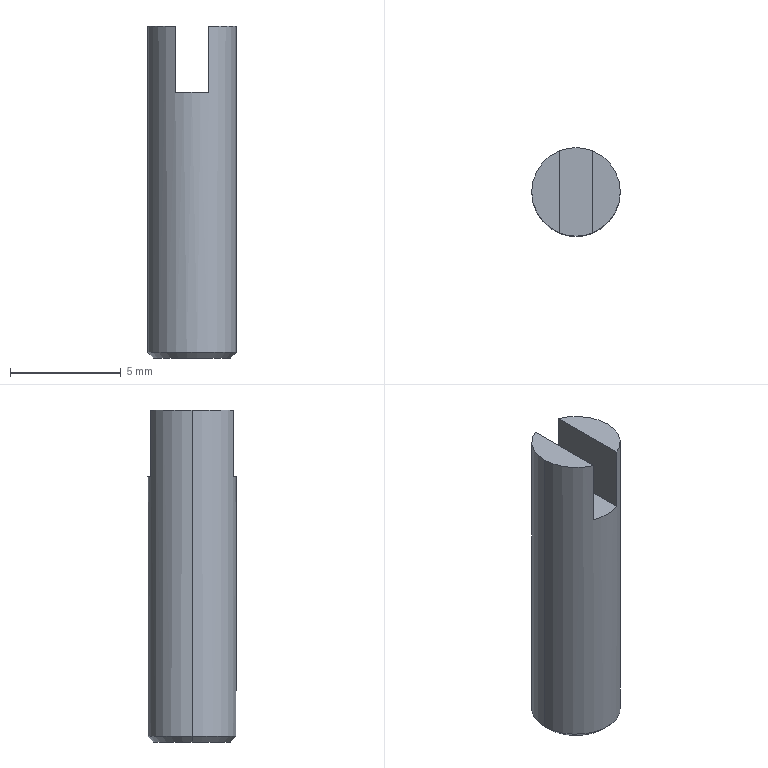Part | SolidWorks | features BaseBody 1 | 1 solid | 10 faces | box 4 x 4 x 15 mm | volume 170.55 mm3 | plane 6 | cone 2 | cylinder 2 | commonest cylinder face diameters 4 x2
STEP:
#1=CARTESIAN_POINT('',(-1.75,0.,0.));
#2=VERTEX_POINT('',#1);
#3=CARTESIAN_POINT('',(1.75,0.,0.));
#4=VERTEX_POINT('',#3);
#5=CARTESIAN_POINT('',(0.,0.,0.));
#6=DIRECTION('',(0.,0.,1.));
#7=DIRECTION('',(-1.,0.,0.));
#8=AXIS2_PLACEMENT_3D('',#5,#6,#7);
#9=CIRCLE('',#8,1.75);
#10=EDGE_CURVE('',#2,#4,#9,.T.);
#11=ORIENTED_EDGE('',*,*,#10,.T.);
#12=CARTESIAN_POINT('',(2.,0.,0.25));
#13=VERTEX_POINT('',#12);
#14=CARTESIAN_POINT('',(1.875,0.,0.125));
#15=DIRECTION('',(0.7071,0.,0.7071));
#16=VECTOR('',#15,1000.);
#17=LINE('',#14,#16);
#18=EDGE_CURVE('',#4,#13,#17,.T.);
#19=ORIENTED_EDGE('',*,*,#18,.T.);
#20=CARTESIAN_POINT('',(-2.,0.,0.25));
#21=VERTEX_POINT('',#20);
#22=CARTESIAN_POINT('',(0.,0.,0.25));
#23=DIRECTION('',(0.,0.,-1.));
#24=DIRECTION('',(-1.,0.,0.));
#25=AXIS2_PLACEMENT_3D('',#22,#23,#24);
#26=CIRCLE('',#25,2.);
#27=EDGE_CURVE('',#13,#21,#26,.T.);
#28=ORIENTED_EDGE('',*,*,#27,.T.);
#29=CARTESIAN_POINT('',(-1.875,0.,0.125));
#30=DIRECTION('',(-0.7071,0.,0.7071));
#31=VECTOR('',#30,1000.);
#32=LINE('',#29,#31);
#33=EDGE_CURVE('',#2,#21,#32,.T.);
#34=ORIENTED_EDGE('',*,*,#33,.F.);
#35=EDGE_LOOP('',(#11,#19,#28,#34));
#36=FACE_OUTER_BOUND('',#35,.T.);
#37=CARTESIAN_POINT('',(0.,0.,0.125));
#38=DIRECTION('',(0.,0.,1.));
#39=DIRECTION('',(-1.,0.,0.));
#40=AXIS2_PLACEMENT_3D('',#37,#38,#39);
#41=CONICAL_SURFACE('',#40,1.875,0.7854);
#42=ADVANCED_FACE('',(#36),#41,.T.);
#43=CARTESIAN_POINT('',(2.,0.,15.));
#44=VERTEX_POINT('',#43);
#45=CARTESIAN_POINT('',(0.75,1.854,15.));
#46=VERTEX_POINT('',#45);
#47=CARTESIAN_POINT('',(0.,0.,15.));
#48=DIRECTION('',(0.,0.,1.));
#49=DIRECTION('',(-1.,0.,0.));
#50=AXIS2_PLACEMENT_3D('',#47,#48,#49);
#51=CIRCLE('',#50,2.);
#52=EDGE_CURVE('',#44,#46,#51,.T.);
#53=ORIENTED_EDGE('',*,*,#52,.F.);
#54=CARTESIAN_POINT('',(2.,0.,0.));
#55=DIRECTION('',(0.,0.,-1.));
#56=VECTOR('',#55,1000.);
#57=LINE('',#54,#56);
#58=EDGE_CURVE('',#44,#13,#57,.T.);
#59=ORIENTED_EDGE('',*,*,#58,.T.);
#60=CARTESIAN_POINT('',(0.,0.,0.25));
#61=DIRECTION('',(0.,0.,-1.));
#62=DIRECTION('',(-1.,0.,0.));
#63=AXIS2_PLACEMENT_3D('',#60,#61,#62);
#64=CIRCLE('',#63,2.);
#65=EDGE_CURVE('',#21,#13,#64,.T.);
#66=ORIENTED_EDGE('',*,*,#65,.F.);
#67=CARTESIAN_POINT('',(-2.,0.,15.));
#68=VERTEX_POINT('',#67);
#69=CARTESIAN_POINT('',(-2.,0.,0.));
#70=DIRECTION('',(0.,0.,-1.));
#71=VECTOR('',#70,1000.);
#72=LINE('',#69,#71);
#73=EDGE_CURVE('',#68,#21,#72,.T.);
#74=ORIENTED_EDGE('',*,*,#73,.F.);
#75=CARTESIAN_POINT('',(-0.75,1.854,15.));
#76=VERTEX_POINT('',#75);
#77=CARTESIAN_POINT('',(0.,0.,15.));
#78=DIRECTION('',(0.,0.,1.));
#79=DIRECTION('',(-1.,0.,0.));
#80=AXIS2_PLACEMENT_3D('',#77,#78,#79);
#81=CIRCLE('',#80,2.);
#82=EDGE_CURVE('',#76,#68,#81,.T.);
#83=ORIENTED_EDGE('',*,*,#82,.F.);
#84=CARTESIAN_POINT('',(-0.75,1.854,12.));
#85=VERTEX_POINT('',#84);
#86=CARTESIAN_POINT('',(-0.75,1.854,0.));
#87=DIRECTION('',(0.,0.,-1.));
#88=VECTOR('',#87,1000.);
#89=LINE('',#86,#88);
#90=EDGE_CURVE('',#76,#85,#89,.T.);
#91=ORIENTED_EDGE('',*,*,#90,.T.);
#92=CARTESIAN_POINT('',(0.75,1.854,12.));
#93=VERTEX_POINT('',#92);
#94=CARTESIAN_POINT('',(0.,0.,12.));
#95=DIRECTION('',(0.,0.,-1.));
#96=DIRECTION('',(-1.,0.,0.));
#97=AXIS2_PLACEMENT_3D('',#94,#95,#96);
#98=CIRCLE('',#97,2.);
#99=EDGE_CURVE('',#85,#93,#98,.T.);
#100=ORIENTED_EDGE('',*,*,#99,.T.);
#101=CARTESIAN_POINT('',(0.75,1.854,0.));
#102=DIRECTION('',(0.,0.,1.));
#103=VECTOR('',#102,1000.);
#104=LINE('',#101,#103);
#105=EDGE_CURVE('',#93,#46,#104,.T.);
#106=ORIENTED_EDGE('',*,*,#105,.T.);
#107=EDGE_LOOP('',(#53,#59,#66,#74,#83,#91,#100,#106));
#108=FACE_OUTER_BOUND('',#107,.T.);
#109=CARTESIAN_POINT('',(0.,0.,0.));
#110=DIRECTION('',(0.,0.,-1.));
#111=DIRECTION('',(-1.,0.,0.));
#112=AXIS2_PLACEMENT_3D('',#109,#110,#111);
#113=CYLINDRICAL_SURFACE('',#112,2.);
#114=ADVANCED_FACE('',(#108),#113,.T.);
#115=ORIENTED_EDGE('',*,*,#10,.F.);
#116=CARTESIAN_POINT('',(0.,0.,0.));
#117=DIRECTION('',(0.,0.,1.));
#118=DIRECTION('',(-1.,0.,0.));
#119=AXIS2_PLACEMENT_3D('',#116,#117,#118);
#120=CIRCLE('',#119,1.75);
#121=EDGE_CURVE('',#4,#2,#120,.T.);
#122=ORIENTED_EDGE('',*,*,#121,.F.);
#123=EDGE_LOOP('',(#115,#122));
#124=FACE_OUTER_BOUND('',#123,.T.);
#125=CARTESIAN_POINT('',(0.,0.,0.));
#126=DIRECTION('',(0.,0.,1.));
#127=DIRECTION('',(1.,0.,0.));
#128=AXIS2_PLACEMENT_3D('',#125,#126,#127);
#129=PLANE('',#128);
#130=ADVANCED_FACE('',(#124),#129,.F.);
#131=CARTESIAN_POINT('',(-0.75,-1.854,12.));
#132=VERTEX_POINT('',#131);
#133=CARTESIAN_POINT('',(-0.75,-1.854,15.));
#134=VERTEX_POINT('',#133);
#135=CARTESIAN_POINT('',(-0.75,-1.854,0.));
#136=DIRECTION('',(0.,0.,1.));
#137=VECTOR('',#136,1000.);
#138=LINE('',#135,#137);
#139=EDGE_CURVE('',#132,#134,#138,.T.);
#140=ORIENTED_EDGE('',*,*,#139,.F.);
#141=CARTESIAN_POINT('',(-0.75,-2.,12.));
#142=DIRECTION('',(0.,1.,0.));
#143=VECTOR('',#142,1000.);
#144=LINE('',#141,#143);
#145=EDGE_CURVE('',#132,#85,#144,.T.);
#146=ORIENTED_EDGE('',*,*,#145,.T.);
#147=ORIENTED_EDGE('',*,*,#90,.F.);
#148=CARTESIAN_POINT('',(-0.75,-1.,15.));
#149=DIRECTION('',(0.,1.,0.));
#150=VECTOR('',#149,1000.);
#151=LINE('',#148,#150);
#152=EDGE_CURVE('',#134,#76,#151,.T.);
#153=ORIENTED_EDGE('',*,*,#152,.F.);
#154=EDGE_LOOP('',(#140,#146,#147,#153));
#155=FACE_OUTER_BOUND('',#154,.T.);
#156=CARTESIAN_POINT('',(-0.75,-2.,15.));
#157=DIRECTION('',(-1.,0.,0.));
#158=DIRECTION('',(0.,1.,0.));
#159=AXIS2_PLACEMENT_3D('',#156,#157,#158);
#160=PLANE('',#159);
#161=ADVANCED_FACE('',(#155),#160,.F.);
#162=CARTESIAN_POINT('',(0.75,-1.854,12.));
#163=VERTEX_POINT('',#162);
#164=CARTESIAN_POINT('',(0.,0.,12.));
#165=DIRECTION('',(0.,0.,-1.));
#166=DIRECTION('',(-1.,0.,0.));
#167=AXIS2_PLACEMENT_3D('',#164,#165,#166);
#168=CIRCLE('',#167,2.);
#169=EDGE_CURVE('',#163,#132,#168,.T.);
#170=ORIENTED_EDGE('',*,*,#169,.F.);
#171=CARTESIAN_POINT('',(0.75,2.,12.));
#172=DIRECTION('',(0.,-1.,0.));
#173=VECTOR('',#172,1000.);
#174=LINE('',#171,#173);
#175=EDGE_CURVE('',#93,#163,#174,.T.);
#176=ORIENTED_EDGE('',*,*,#175,.F.);
#177=ORIENTED_EDGE('',*,*,#99,.F.);
#178=ORIENTED_EDGE('',*,*,#145,.F.);
#179=EDGE_LOOP('',(#170,#176,#177,#178));
#180=FACE_OUTER_BOUND('',#179,.T.);
#181=CARTESIAN_POINT('',(0.,0.,12.));
#182=DIRECTION('',(0.,0.,-1.));
#183=DIRECTION('',(0.,-1.,0.));
#184=AXIS2_PLACEMENT_3D('',#181,#182,#183);
#185=PLANE('',#184);
#186=ADVANCED_FACE('',(#180),#185,.F.);
#187=CARTESIAN_POINT('',(0.75,-1.854,15.));
#188=VERTEX_POINT('',#187);
#189=CARTESIAN_POINT('',(0.75,-1.854,0.));
#190=DIRECTION('',(0.,0.,-1.));
#191=VECTOR('',#190,1000.);
#192=LINE('',#189,#191);
#193=EDGE_CURVE('',#188,#163,#192,.T.);
#194=ORIENTED_EDGE('',*,*,#193,.F.);
#195=CARTESIAN_POINT('',(0.75,1.,15.));
#196=DIRECTION('',(0.,-1.,0.));
#197=VECTOR('',#196,1000.);
#198=LINE('',#195,#197);
#199=EDGE_CURVE('',#46,#188,#198,.T.);
#200=ORIENTED_EDGE('',*,*,#199,.F.);
#201=ORIENTED_EDGE('',*,*,#105,.F.);
#202=ORIENTED_EDGE('',*,*,#175,.T.);
#203=EDGE_LOOP('',(#194,#200,#201,#202));
#204=FACE_OUTER_BOUND('',#203,.T.);
#205=CARTESIAN_POINT('',(0.75,2.,15.));
#206=DIRECTION('',(1.,0.,0.));
#207=DIRECTION('',(0.,-1.,0.));
#208=AXIS2_PLACEMENT_3D('',#205,#206,#207);
#209=PLANE('',#208);
#210=ADVANCED_FACE('',(#204),#209,.F.);
#211=ORIENTED_EDGE('',*,*,#152,.T.);
#212=ORIENTED_EDGE('',*,*,#82,.T.);
#213=CARTESIAN_POINT('',(0.,0.,15.));
#214=DIRECTION('',(0.,0.,1.));
#215=DIRECTION('',(-1.,0.,0.));
#216=AXIS2_PLACEMENT_3D('',#213,#214,#215);
#217=CIRCLE('',#216,2.);
#218=EDGE_CURVE('',#68,#134,#217,.T.);
#219=ORIENTED_EDGE('',*,*,#218,.T.);
#220=EDGE_LOOP('',(#211,#212,#219));
#221=FACE_OUTER_BOUND('',#220,.T.);
#222=CARTESIAN_POINT('',(0.,0.,15.));
#223=DIRECTION('',(0.,0.,1.));
#224=DIRECTION('',(1.,0.,0.));
#225=AXIS2_PLACEMENT_3D('',#222,#223,#224);
#226=PLANE('',#225);
#227=ADVANCED_FACE('',(#221),#226,.T.);
#228=ORIENTED_EDGE('',*,*,#199,.T.);
#229=CARTESIAN_POINT('',(0.,0.,15.));
#230=DIRECTION('',(0.,0.,1.));
#231=DIRECTION('',(-1.,0.,0.));
#232=AXIS2_PLACEMENT_3D('',#229,#230,#231);
#233=CIRCLE('',#232,2.);
#234=EDGE_CURVE('',#188,#44,#233,.T.);
#235=ORIENTED_EDGE('',*,*,#234,.T.);
#236=ORIENTED_EDGE('',*,*,#52,.T.);
#237=EDGE_LOOP('',(#228,#235,#236));
#238=FACE_OUTER_BOUND('',#237,.T.);
#239=CARTESIAN_POINT('',(0.,0.,15.));
#240=DIRECTION('',(0.,0.,1.));
#241=DIRECTION('',(1.,0.,0.));
#242=AXIS2_PLACEMENT_3D('',#239,#240,#241);
#243=PLANE('',#242);
#244=ADVANCED_FACE('',(#238),#243,.T.);
#245=ORIENTED_EDGE('',*,*,#58,.F.);
#246=ORIENTED_EDGE('',*,*,#234,.F.);
#247=ORIENTED_EDGE('',*,*,#193,.T.);
#248=ORIENTED_EDGE('',*,*,#169,.T.);
#249=ORIENTED_EDGE('',*,*,#139,.T.);
#250=ORIENTED_EDGE('',*,*,#218,.F.);
#251=ORIENTED_EDGE('',*,*,#73,.T.);
#252=ORIENTED_EDGE('',*,*,#27,.F.);
#253=EDGE_LOOP('',(#245,#246,#247,#248,#249,#250,#251,#252));
#254=FACE_OUTER_BOUND('',#253,.T.);
#255=CARTESIAN_POINT('',(0.,0.,0.));
#256=DIRECTION('',(0.,0.,-1.));
#257=DIRECTION('',(-1.,0.,0.));
#258=AXIS2_PLACEMENT_3D('',#255,#256,#257);
#259=CYLINDRICAL_SURFACE('',#258,2.);
#260=ADVANCED_FACE('',(#254),#259,.T.);
#261=ORIENTED_EDGE('',*,*,#18,.F.);
#262=ORIENTED_EDGE('',*,*,#121,.T.);
#263=ORIENTED_EDGE('',*,*,#33,.T.);
#264=ORIENTED_EDGE('',*,*,#65,.T.);
#265=EDGE_LOOP('',(#261,#262,#263,#264));
#266=FACE_OUTER_BOUND('',#265,.T.);
#267=CARTESIAN_POINT('',(0.,0.,0.125));
#268=DIRECTION('',(0.,0.,1.));
#269=DIRECTION('',(-1.,0.,0.));
#270=AXIS2_PLACEMENT_3D('',#267,#268,#269);
#271=CONICAL_SURFACE('',#270,1.875,0.7854);
#272=ADVANCED_FACE('',(#266),#271,.T.);
#273=CLOSED_SHELL('',(#42,#114,#130,#161,#186,#210,#227,#244,#260,#272));
#274=MANIFOLD_SOLID_BREP('',#273);
#275=CARTESIAN_POINT('',(0.,0.,0.));
#276=DIRECTION('',(0.,0.,1.));
#277=DIRECTION('',(1.,0.,0.));
#278=AXIS2_PLACEMENT_3D('',#275,#276,#277);
#279=(LENGTH_UNIT()NAMED_UNIT(*)SI_UNIT(.MILLI.,.METRE.));
#280=UNCERTAINTY_MEASURE_WITH_UNIT(LENGTH_MEASURE(0.00001),#279,'','');
#281=(NAMED_UNIT(*)PLANE_ANGLE_UNIT()SI_UNIT($,.RADIAN.));
#282=(NAMED_UNIT(*)SI_UNIT($,.STERADIAN.)SOLID_ANGLE_UNIT());
#283=(GEOMETRIC_REPRESENTATION_CONTEXT(3)GLOBAL_UNCERTAINTY_ASSIGNED_CONTEXT((#280))GLOBAL_UNIT_ASSIGNED_CONTEXT((#279,#281,#282))REPRESENTATION_CONTEXT('',''));
#284=ADVANCED_BREP_SHAPE_REPRESENTATION('',(#274,#278),#283);